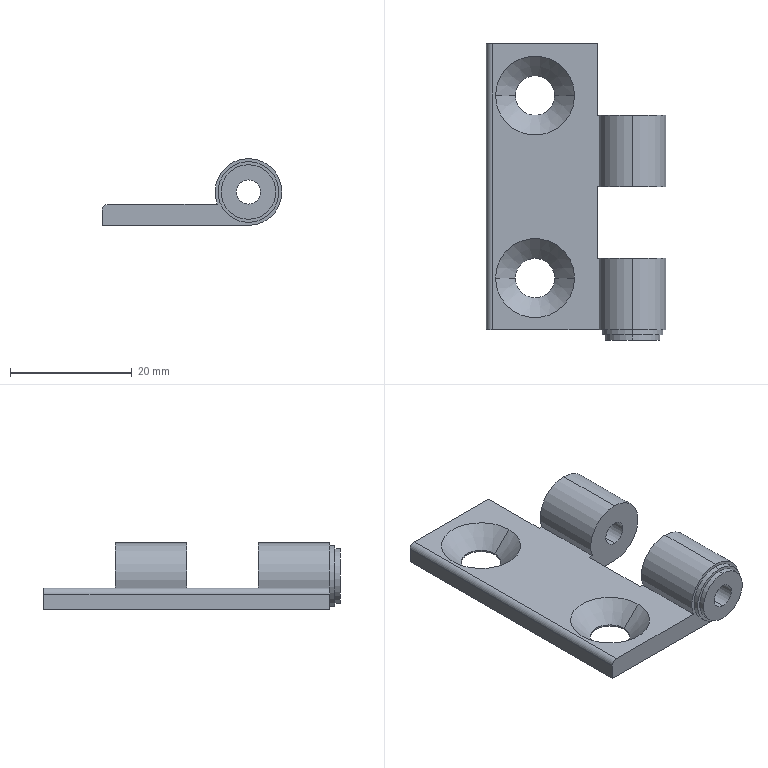Part | STEP file | 1 solid | 33 faces | box 29.5 x 48.7 x 11 mm | volume 4677 mm3 | cylinder 17 | plane 12 | cone 4 | commonest cylinder face diameters 4 x4 6.5 x4 11 x4 9 x2 10 x2 2 x1